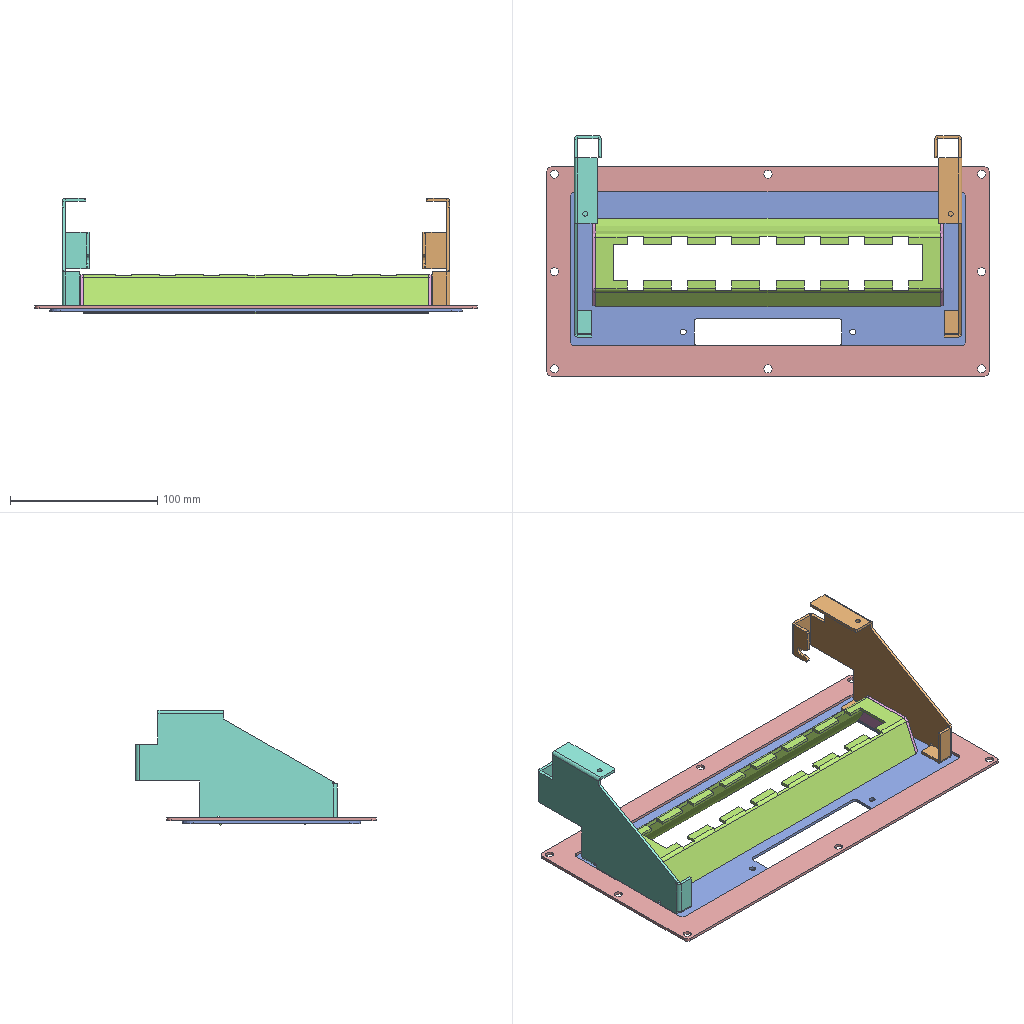Assembly | SolidWorks | 6 different items | 7 placed | box 300 x 163 x 78 mm
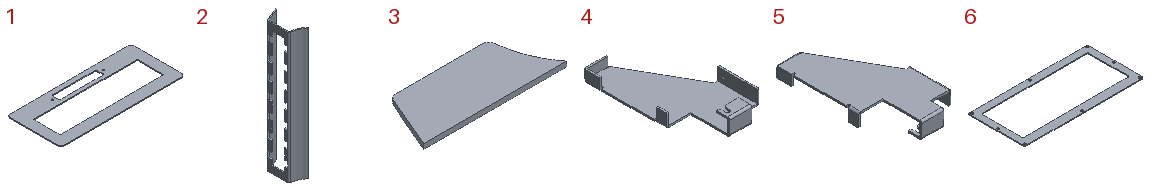Parts list (item | quantity | size | volume | features):
1 | x1 | 280 x 121 x 2 mm | 35940 mm3 | features FlatPattern 1, SMBaseFlange 1, SheetMetal 1
2 | x1 | 26.364 x 60 x 234 mm | 30210 mm3 | features FlatPattern 1, ICE 1, SMBaseFlange 1, SheetMetal 1
3 | x2 | 57.397 x 23 x 2 mm | 2146 mm3 | features FlatPattern 1, SMBaseFlange 1, SheetMetal 1
4 | x1 | 75 x 136.5 x 18.5 mm | 16677 mm3 | features EdgeFlange 6, ICE 2, Fillet 1, FlatPattern 1, SMBaseFlange 1, SheetMetal 1
5 | x1 | 75 x 136.5 x 18.5 mm | 16677 mm3 | features MirrorStock 1
6 | x1 | 300 x 142 x 2 mm | 28808 mm3 | features FlatPattern 1, SMBaseFlange 1, SheetMetal 1
Mates (type | each side: item.copy, entity, surface, feature):
Coincident | 6.1 face plane Base-Flange1 | 1.1 face plane Base-Flange1
DistanceDim | 1.1 face plane Base-Flange1 | 6.1 face plane Base-Flange1 | 2 times
Concentric | 2.1 face cylinder Base Bend1 | 3.1 face cylinder Base-Flange1
Parallel | 2.1 face plane Base-Flange1 | 3.1 face plane Base-Flange1
Coincident | 2.1 face plane Base Bend1 | 3.1 face plane Base-Flange1
Coincident | 2.1 face plane Base Bend1 | 3.2 face plane Base-Flange1
Coincident | 2.1 face plane Base-Flange1 | 3.2 face plane Base-Flange1 | 2 times
Coincident | 1.1 face plane Base-Flange1 | 3.2 face plane Base-Flange1
Coincident | 1.1 face plane Base-Flange1 | 2.1 face plane Base-Flange1
Coincident | 1.1 edge | 2.1 edge
Coincident | 1.1 face plane Base-Flange1 | 4.1 face plane Edge-Flange2
DistanceDim | 4.1 face plane Base-Flange1 | 6.1 face plane Base-Flange1
DistanceDim | 4.1 face plane Edge-Flange1 | 6.1 face plane Base-Flange1